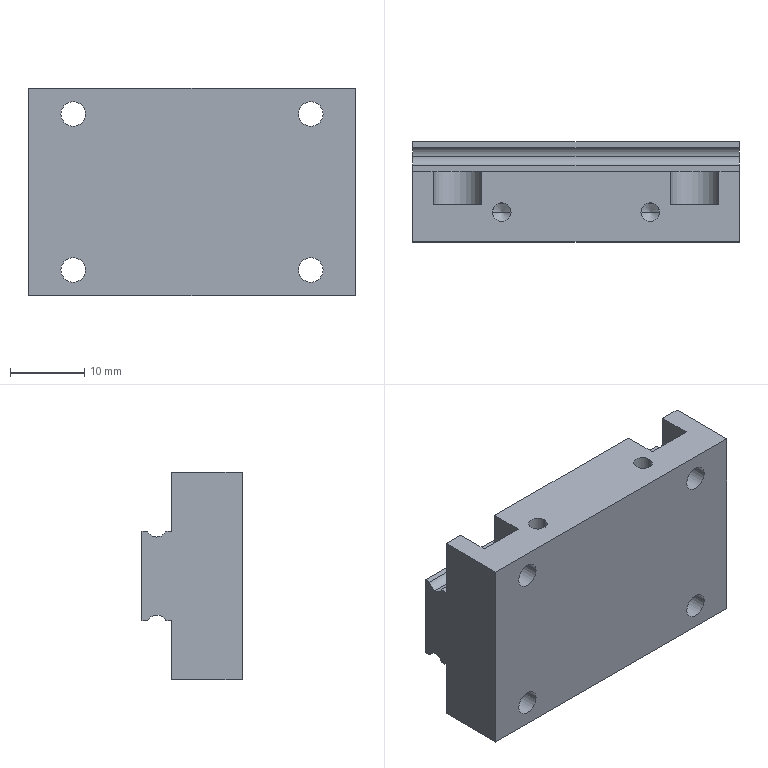Part | NX | 1 solid | 55 faces | box 44 x 13.5 x 28 mm | volume 12700 mm3 | plane 24 | cylinder 23 | cone 8 | commonest cylinder face diameters 2.5 x8 3.3 x8 6.5 x4 2.7 x3